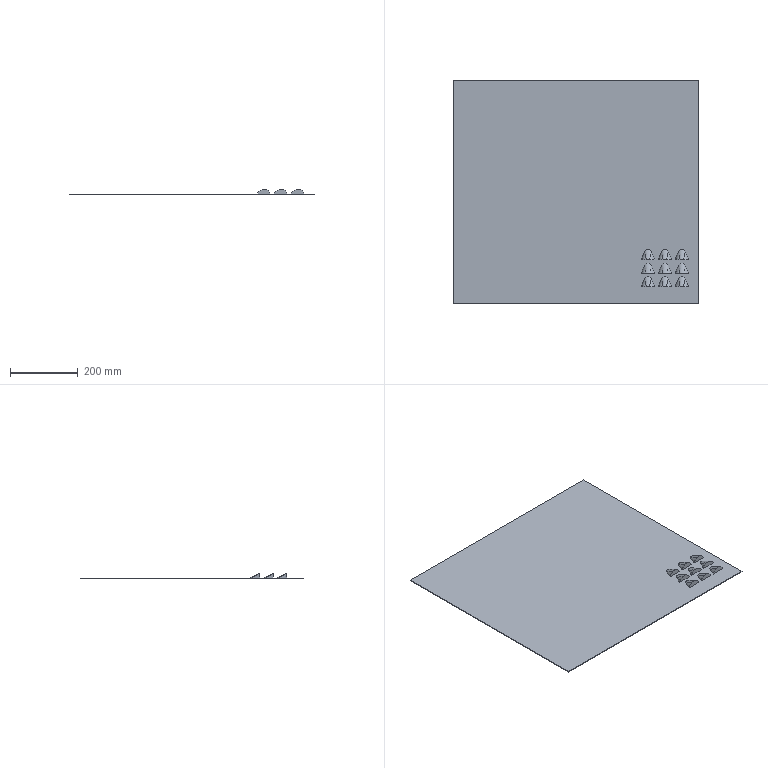Part | SolidWorks | features BaseBody 1 | 1 solid | 42 faces | box 724 x 660 x 17 mm | volume 998776 mm3 | spline 27 | plane 15